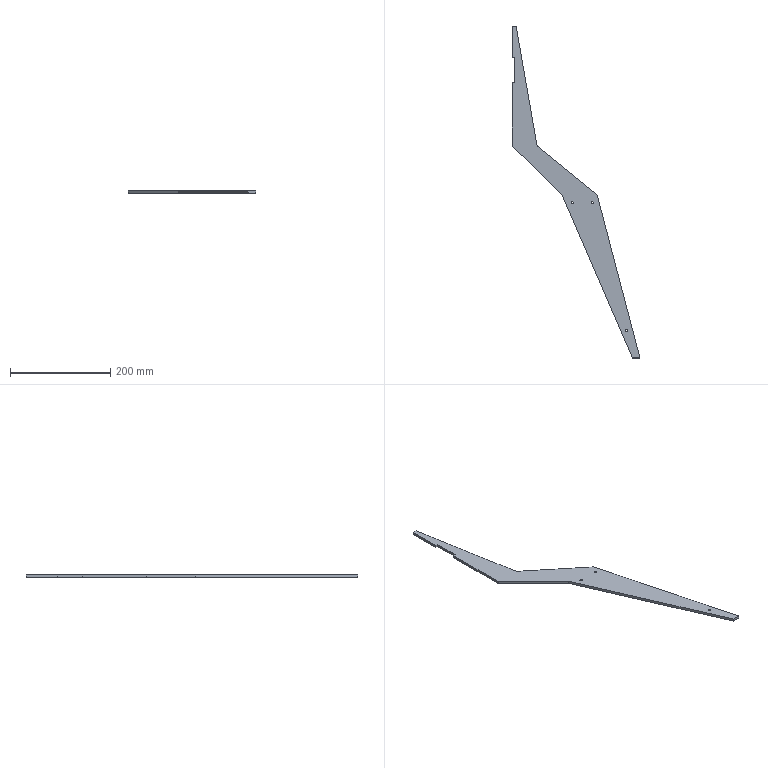Part | SolidWorks | features Cut 1, Extrusion 1, ICE 1 | 1 solid | 20 faces | box 255 x 663 x 5 mm | volume 131784 mm3 | plane 14 | cylinder 6 | commonest cylinder face diameters 4.4 x6
STEP:
#1=CARTESIAN_POINT('',(230.662,-608.,-2.5));
#2=VERTEX_POINT('',#1);
#3=CARTESIAN_POINT('',(226.262,-608.,-2.5));
#4=VERTEX_POINT('',#3);
#5=CARTESIAN_POINT('',(228.462,-608.,-2.5));
#6=DIRECTION('',(0.,0.,-1.));
#7=DIRECTION('',(-1.,0.,0.));
#8=AXIS2_PLACEMENT_3D('',#5,#6,#7);
#9=CIRCLE('',#8,2.2);
#10=EDGE_CURVE('',#2,#4,#9,.T.);
#11=ORIENTED_EDGE('',*,*,#10,.T.);
#12=CARTESIAN_POINT('',(226.262,-608.,2.5));
#13=VERTEX_POINT('',#12);
#14=CARTESIAN_POINT('',(226.262,-608.,-7.5));
#15=DIRECTION('',(0.,0.,1.));
#16=VECTOR('',#15,1000.);
#17=LINE('',#14,#16);
#18=EDGE_CURVE('',#4,#13,#17,.T.);
#19=ORIENTED_EDGE('',*,*,#18,.T.);
#20=CARTESIAN_POINT('',(230.662,-608.,2.5));
#21=VERTEX_POINT('',#20);
#22=CARTESIAN_POINT('',(228.462,-608.,2.5));
#23=DIRECTION('',(0.,0.,1.));
#24=DIRECTION('',(1.,0.,0.));
#25=AXIS2_PLACEMENT_3D('',#22,#23,#24);
#26=CIRCLE('',#25,2.2);
#27=EDGE_CURVE('',#13,#21,#26,.T.);
#28=ORIENTED_EDGE('',*,*,#27,.T.);
#29=CARTESIAN_POINT('',(230.662,-608.,-7.5));
#30=DIRECTION('',(0.,0.,1.));
#31=VECTOR('',#30,1000.);
#32=LINE('',#29,#31);
#33=EDGE_CURVE('',#2,#21,#32,.T.);
#34=ORIENTED_EDGE('',*,*,#33,.F.);
#35=EDGE_LOOP('',(#11,#19,#28,#34));
#36=FACE_OUTER_BOUND('',#35,.T.);
#37=CARTESIAN_POINT('',(228.462,-608.,-7.5));
#38=DIRECTION('',(0.,0.,1.));
#39=DIRECTION('',(1.,0.,0.));
#40=AXIS2_PLACEMENT_3D('',#37,#38,#39);
#41=CYLINDRICAL_SURFACE('',#40,2.2);
#42=ADVANCED_FACE('',(#36),#41,.F.);
#43=CARTESIAN_POINT('',(122.392,-353.,-2.5));
#44=VERTEX_POINT('',#43);
#45=CARTESIAN_POINT('',(117.992,-353.,-2.5));
#46=VERTEX_POINT('',#45);
#47=CARTESIAN_POINT('',(120.192,-353.,-2.5));
#48=DIRECTION('',(0.,0.,-1.));
#49=DIRECTION('',(-1.,0.,0.));
#50=AXIS2_PLACEMENT_3D('',#47,#48,#49);
#51=CIRCLE('',#50,2.2);
#52=EDGE_CURVE('',#44,#46,#51,.T.);
#53=ORIENTED_EDGE('',*,*,#52,.T.);
#54=CARTESIAN_POINT('',(117.992,-353.,2.5));
#55=VERTEX_POINT('',#54);
#56=CARTESIAN_POINT('',(117.992,-353.,-7.5));
#57=DIRECTION('',(0.,0.,1.));
#58=VECTOR('',#57,1000.);
#59=LINE('',#56,#58);
#60=EDGE_CURVE('',#46,#55,#59,.T.);
#61=ORIENTED_EDGE('',*,*,#60,.T.);
#62=CARTESIAN_POINT('',(122.392,-353.,2.5));
#63=VERTEX_POINT('',#62);
#64=CARTESIAN_POINT('',(120.192,-353.,2.5));
#65=DIRECTION('',(0.,0.,1.));
#66=DIRECTION('',(1.,0.,0.));
#67=AXIS2_PLACEMENT_3D('',#64,#65,#66);
#68=CIRCLE('',#67,2.2);
#69=EDGE_CURVE('',#55,#63,#68,.T.);
#70=ORIENTED_EDGE('',*,*,#69,.T.);
#71=CARTESIAN_POINT('',(122.392,-353.,-7.5));
#72=DIRECTION('',(0.,0.,1.));
#73=VECTOR('',#72,1000.);
#74=LINE('',#71,#73);
#75=EDGE_CURVE('',#44,#63,#74,.T.);
#76=ORIENTED_EDGE('',*,*,#75,.F.);
#77=EDGE_LOOP('',(#53,#61,#70,#76));
#78=FACE_OUTER_BOUND('',#77,.T.);
#79=CARTESIAN_POINT('',(120.192,-353.,-7.5));
#80=DIRECTION('',(0.,0.,1.));
#81=DIRECTION('',(1.,0.,0.));
#82=AXIS2_PLACEMENT_3D('',#79,#80,#81);
#83=CYLINDRICAL_SURFACE('',#82,2.2);
#84=ADVANCED_FACE('',(#78),#83,.F.);
#85=CARTESIAN_POINT('',(162.392,-353.,-2.5));
#86=VERTEX_POINT('',#85);
#87=CARTESIAN_POINT('',(157.992,-353.,-2.5));
#88=VERTEX_POINT('',#87);
#89=CARTESIAN_POINT('',(160.192,-353.,-2.5));
#90=DIRECTION('',(0.,0.,-1.));
#91=DIRECTION('',(-1.,0.,0.));
#92=AXIS2_PLACEMENT_3D('',#89,#90,#91);
#93=CIRCLE('',#92,2.2);
#94=EDGE_CURVE('',#86,#88,#93,.T.);
#95=ORIENTED_EDGE('',*,*,#94,.T.);
#96=CARTESIAN_POINT('',(157.992,-353.,2.5));
#97=VERTEX_POINT('',#96);
#98=CARTESIAN_POINT('',(157.992,-353.,-7.5));
#99=DIRECTION('',(0.,0.,1.));
#100=VECTOR('',#99,1000.);
#101=LINE('',#98,#100);
#102=EDGE_CURVE('',#88,#97,#101,.T.);
#103=ORIENTED_EDGE('',*,*,#102,.T.);
#104=CARTESIAN_POINT('',(162.392,-353.,2.5));
#105=VERTEX_POINT('',#104);
#106=CARTESIAN_POINT('',(160.192,-353.,2.5));
#107=DIRECTION('',(0.,0.,1.));
#108=DIRECTION('',(1.,0.,0.));
#109=AXIS2_PLACEMENT_3D('',#106,#107,#108);
#110=CIRCLE('',#109,2.2);
#111=EDGE_CURVE('',#97,#105,#110,.T.);
#112=ORIENTED_EDGE('',*,*,#111,.T.);
#113=CARTESIAN_POINT('',(162.392,-353.,-7.5));
#114=DIRECTION('',(0.,0.,1.));
#115=VECTOR('',#114,1000.);
#116=LINE('',#113,#115);
#117=EDGE_CURVE('',#86,#105,#116,.T.);
#118=ORIENTED_EDGE('',*,*,#117,.F.);
#119=EDGE_LOOP('',(#95,#103,#112,#118));
#120=FACE_OUTER_BOUND('',#119,.T.);
#121=CARTESIAN_POINT('',(160.192,-353.,-7.5));
#122=DIRECTION('',(0.,0.,1.));
#123=DIRECTION('',(1.,0.,0.));
#124=AXIS2_PLACEMENT_3D('',#121,#122,#123);
#125=CYLINDRICAL_SURFACE('',#124,2.2);
#126=ADVANCED_FACE('',(#120),#125,.F.);
#127=CARTESIAN_POINT('',(0.,0.,-2.5));
#128=VERTEX_POINT('',#127);
#129=CARTESIAN_POINT('',(0.,-63.,-2.5));
#130=VERTEX_POINT('',#129);
#131=CARTESIAN_POINT('',(0.,-63.,-2.5));
#132=DIRECTION('',(0.,-1.,0.));
#133=VECTOR('',#132,1000.);
#134=LINE('',#131,#133);
#135=EDGE_CURVE('',#128,#130,#134,.T.);
#136=ORIENTED_EDGE('',*,*,#135,.T.);
#137=CARTESIAN_POINT('',(0.,-63.,2.5));
#138=VERTEX_POINT('',#137);
#139=CARTESIAN_POINT('',(0.,-63.,2.5));
#140=DIRECTION('',(0.,0.,-1.));
#141=VECTOR('',#140,1000.);
#142=LINE('',#139,#141);
#143=EDGE_CURVE('',#138,#130,#142,.T.);
#144=ORIENTED_EDGE('',*,*,#143,.F.);
#145=CARTESIAN_POINT('',(0.,0.,2.5));
#146=VERTEX_POINT('',#145);
#147=CARTESIAN_POINT('',(0.,-63.,2.5));
#148=DIRECTION('',(0.,-1.,0.));
#149=VECTOR('',#148,1000.);
#150=LINE('',#147,#149);
#151=EDGE_CURVE('',#146,#138,#150,.T.);
#152=ORIENTED_EDGE('',*,*,#151,.F.);
#153=CARTESIAN_POINT('',(0.,0.,2.5));
#154=DIRECTION('',(0.,0.,-1.));
#155=VECTOR('',#154,1000.);
#156=LINE('',#153,#155);
#157=EDGE_CURVE('',#146,#128,#156,.T.);
#158=ORIENTED_EDGE('',*,*,#157,.T.);
#159=EDGE_LOOP('',(#136,#144,#152,#158));
#160=FACE_OUTER_BOUND('',#159,.T.);
#161=CARTESIAN_POINT('',(0.,-63.,2.5));
#162=DIRECTION('',(1.,0.,0.));
#163=DIRECTION('',(0.,0.,-1.));
#164=AXIS2_PLACEMENT_3D('',#161,#162,#163);
#165=PLANE('',#164);
#166=ADVANCED_FACE('',(#160),#165,.F.);
#167=CARTESIAN_POINT('',(5.,-63.,-2.5));
#168=VERTEX_POINT('',#167);
#169=CARTESIAN_POINT('',(5.,-63.,-2.5));
#170=DIRECTION('',(1.,0.,0.));
#171=VECTOR('',#170,1000.);
#172=LINE('',#169,#171);
#173=EDGE_CURVE('',#130,#168,#172,.T.);
#174=ORIENTED_EDGE('',*,*,#173,.T.);
#175=CARTESIAN_POINT('',(5.,-63.,2.5));
#176=VERTEX_POINT('',#175);
#177=CARTESIAN_POINT('',(5.,-63.,2.5));
#178=DIRECTION('',(0.,0.,-1.));
#179=VECTOR('',#178,1000.);
#180=LINE('',#177,#179);
#181=EDGE_CURVE('',#176,#168,#180,.T.);
#182=ORIENTED_EDGE('',*,*,#181,.F.);
#183=CARTESIAN_POINT('',(5.,-63.,2.5));
#184=DIRECTION('',(1.,0.,0.));
#185=VECTOR('',#184,1000.);
#186=LINE('',#183,#185);
#187=EDGE_CURVE('',#138,#176,#186,.T.);
#188=ORIENTED_EDGE('',*,*,#187,.F.);
#189=ORIENTED_EDGE('',*,*,#143,.T.);
#190=EDGE_LOOP('',(#174,#182,#188,#189));
#191=FACE_OUTER_BOUND('',#190,.T.);
#192=CARTESIAN_POINT('',(5.,-63.,2.5));
#193=DIRECTION('',(0.,1.,0.));
#194=DIRECTION('',(0.,0.,1.));
#195=AXIS2_PLACEMENT_3D('',#192,#193,#194);
#196=PLANE('',#195);
#197=ADVANCED_FACE('',(#191),#196,.F.);
#198=CARTESIAN_POINT('',(5.,-113.,-2.5));
#199=VERTEX_POINT('',#198);
#200=CARTESIAN_POINT('',(5.,-113.,-2.5));
#201=DIRECTION('',(0.,-1.,0.));
#202=VECTOR('',#201,1000.);
#203=LINE('',#200,#202);
#204=EDGE_CURVE('',#168,#199,#203,.T.);
#205=ORIENTED_EDGE('',*,*,#204,.T.);
#206=CARTESIAN_POINT('',(5.,-113.,2.5));
#207=VERTEX_POINT('',#206);
#208=CARTESIAN_POINT('',(5.,-113.,2.5));
#209=DIRECTION('',(0.,0.,-1.));
#210=VECTOR('',#209,1000.);
#211=LINE('',#208,#210);
#212=EDGE_CURVE('',#207,#199,#211,.T.);
#213=ORIENTED_EDGE('',*,*,#212,.F.);
#214=CARTESIAN_POINT('',(5.,-113.,2.5));
#215=DIRECTION('',(0.,-1.,0.));
#216=VECTOR('',#215,1000.);
#217=LINE('',#214,#216);
#218=EDGE_CURVE('',#176,#207,#217,.T.);
#219=ORIENTED_EDGE('',*,*,#218,.F.);
#220=ORIENTED_EDGE('',*,*,#181,.T.);
#221=EDGE_LOOP('',(#205,#213,#219,#220));
#222=FACE_OUTER_BOUND('',#221,.T.);
#223=CARTESIAN_POINT('',(5.,-113.,2.5));
#224=DIRECTION('',(1.,0.,0.));
#225=DIRECTION('',(0.,0.,-1.));
#226=AXIS2_PLACEMENT_3D('',#223,#224,#225);
#227=PLANE('',#226);
#228=ADVANCED_FACE('',(#222),#227,.F.);
#229=CARTESIAN_POINT('',(0.,-113.,-2.5));
#230=VERTEX_POINT('',#229);
#231=CARTESIAN_POINT('',(0.,-113.,-2.5));
#232=DIRECTION('',(-1.,0.,0.));
#233=VECTOR('',#232,1000.);
#234=LINE('',#231,#233);
#235=EDGE_CURVE('',#199,#230,#234,.T.);
#236=ORIENTED_EDGE('',*,*,#235,.T.);
#237=CARTESIAN_POINT('',(0.,-113.,2.5));
#238=VERTEX_POINT('',#237);
#239=CARTESIAN_POINT('',(0.,-113.,2.5));
#240=DIRECTION('',(0.,0.,-1.));
#241=VECTOR('',#240,1000.);
#242=LINE('',#239,#241);
#243=EDGE_CURVE('',#238,#230,#242,.T.);
#244=ORIENTED_EDGE('',*,*,#243,.F.);
#245=CARTESIAN_POINT('',(0.,-113.,2.5));
#246=DIRECTION('',(-1.,0.,0.));
#247=VECTOR('',#246,1000.);
#248=LINE('',#245,#247);
#249=EDGE_CURVE('',#207,#238,#248,.T.);
#250=ORIENTED_EDGE('',*,*,#249,.F.);
#251=ORIENTED_EDGE('',*,*,#212,.T.);
#252=EDGE_LOOP('',(#236,#244,#250,#251));
#253=FACE_OUTER_BOUND('',#252,.T.);
#254=CARTESIAN_POINT('',(0.,-113.,2.5));
#255=DIRECTION('',(0.,-1.,0.));
#256=DIRECTION('',(0.,0.,-1.));
#257=AXIS2_PLACEMENT_3D('',#254,#255,#256);
#258=PLANE('',#257);
#259=ADVANCED_FACE('',(#253),#258,.F.);
#260=CARTESIAN_POINT('',(0.,-240.,-2.5));
#261=VERTEX_POINT('',#260);
#262=CARTESIAN_POINT('',(0.,-240.,-2.5));
#263=DIRECTION('',(0.,-1.,0.));
#264=VECTOR('',#263,1000.);
#265=LINE('',#262,#264);
#266=EDGE_CURVE('',#230,#261,#265,.T.);
#267=ORIENTED_EDGE('',*,*,#266,.T.);
#268=CARTESIAN_POINT('',(0.,-240.,2.5));
#269=VERTEX_POINT('',#268);
#270=CARTESIAN_POINT('',(0.,-240.,2.5));
#271=DIRECTION('',(0.,0.,-1.));
#272=VECTOR('',#271,1000.);
#273=LINE('',#270,#272);
#274=EDGE_CURVE('',#269,#261,#273,.T.);
#275=ORIENTED_EDGE('',*,*,#274,.F.);
#276=CARTESIAN_POINT('',(0.,-240.,2.5));
#277=DIRECTION('',(0.,-1.,0.));
#278=VECTOR('',#277,1000.);
#279=LINE('',#276,#278);
#280=EDGE_CURVE('',#238,#269,#279,.T.);
#281=ORIENTED_EDGE('',*,*,#280,.F.);
#282=ORIENTED_EDGE('',*,*,#243,.T.);
#283=EDGE_LOOP('',(#267,#275,#281,#282));
#284=FACE_OUTER_BOUND('',#283,.T.);
#285=CARTESIAN_POINT('',(0.,-240.,2.5));
#286=DIRECTION('',(1.,0.,0.));
#287=DIRECTION('',(0.,0.,-1.));
#288=AXIS2_PLACEMENT_3D('',#285,#286,#287);
#289=PLANE('',#288);
#290=ADVANCED_FACE('',(#284),#289,.F.);
#291=CARTESIAN_POINT('',(100.,-338.,-2.5));
#292=VERTEX_POINT('',#291);
#293=CARTESIAN_POINT('',(100.,-338.,-2.5));
#294=DIRECTION('',(0.7142,-0.6999,0.));
#295=VECTOR('',#294,1000.);
#296=LINE('',#293,#295);
#297=EDGE_CURVE('',#261,#292,#296,.T.);
#298=ORIENTED_EDGE('',*,*,#297,.T.);
#299=CARTESIAN_POINT('',(100.,-338.,2.5));
#300=VERTEX_POINT('',#299);
#301=CARTESIAN_POINT('',(100.,-338.,2.5));
#302=DIRECTION('',(0.,0.,-1.));
#303=VECTOR('',#302,1000.);
#304=LINE('',#301,#303);
#305=EDGE_CURVE('',#300,#292,#304,.T.);
#306=ORIENTED_EDGE('',*,*,#305,.F.);
#307=CARTESIAN_POINT('',(100.,-338.,2.5));
#308=DIRECTION('',(0.7142,-0.6999,0.));
#309=VECTOR('',#308,1000.);
#310=LINE('',#307,#309);
#311=EDGE_CURVE('',#269,#300,#310,.T.);
#312=ORIENTED_EDGE('',*,*,#311,.F.);
#313=ORIENTED_EDGE('',*,*,#274,.T.);
#314=EDGE_LOOP('',(#298,#306,#312,#313));
#315=FACE_OUTER_BOUND('',#314,.T.);
#316=CARTESIAN_POINT('',(100.,-338.,2.5));
#317=DIRECTION('',(0.6999,0.7142,0.));
#318=DIRECTION('',(-0.7142,0.6999,0.));
#319=AXIS2_PLACEMENT_3D('',#316,#317,#318);
#320=PLANE('',#319);
#321=ADVANCED_FACE('',(#315),#320,.F.);
#322=CARTESIAN_POINT('',(240.,-663.,-2.5));
#323=VERTEX_POINT('',#322);
#324=CARTESIAN_POINT('',(240.,-663.,-2.5));
#325=DIRECTION('',(0.3956,-0.9184,0.));
#326=VECTOR('',#325,1000.);
#327=LINE('',#324,#326);
#328=EDGE_CURVE('',#292,#323,#327,.T.);
#329=ORIENTED_EDGE('',*,*,#328,.T.);
#330=CARTESIAN_POINT('',(240.,-663.,2.5));
#331=VERTEX_POINT('',#330);
#332=CARTESIAN_POINT('',(240.,-663.,2.5));
#333=DIRECTION('',(0.,0.,-1.));
#334=VECTOR('',#333,1000.);
#335=LINE('',#332,#334);
#336=EDGE_CURVE('',#331,#323,#335,.T.);
#337=ORIENTED_EDGE('',*,*,#336,.F.);
#338=CARTESIAN_POINT('',(240.,-663.,2.5));
#339=DIRECTION('',(0.3956,-0.9184,0.));
#340=VECTOR('',#339,1000.);
#341=LINE('',#338,#340);
#342=EDGE_CURVE('',#300,#331,#341,.T.);
#343=ORIENTED_EDGE('',*,*,#342,.F.);
#344=ORIENTED_EDGE('',*,*,#305,.T.);
#345=EDGE_LOOP('',(#329,#337,#343,#344));
#346=FACE_OUTER_BOUND('',#345,.T.);
#347=CARTESIAN_POINT('',(240.,-663.,2.5));
#348=DIRECTION('',(0.9184,0.3956,0.));
#349=DIRECTION('',(-0.3956,0.9184,0.));
#350=AXIS2_PLACEMENT_3D('',#347,#348,#349);
#351=PLANE('',#350);
#352=ADVANCED_FACE('',(#346),#351,.F.);
#353=CARTESIAN_POINT('',(255.,-663.,-2.5));
#354=VERTEX_POINT('',#353);
#355=CARTESIAN_POINT('',(255.,-663.,-2.5));
#356=DIRECTION('',(1.,0.,0.));
#357=VECTOR('',#356,1000.);
#358=LINE('',#355,#357);
#359=EDGE_CURVE('',#323,#354,#358,.T.);
#360=ORIENTED_EDGE('',*,*,#359,.T.);
#361=CARTESIAN_POINT('',(255.,-663.,2.5));
#362=VERTEX_POINT('',#361);
#363=CARTESIAN_POINT('',(255.,-663.,2.5));
#364=DIRECTION('',(0.,0.,-1.));
#365=VECTOR('',#364,1000.);
#366=LINE('',#363,#365);
#367=EDGE_CURVE('',#362,#354,#366,.T.);
#368=ORIENTED_EDGE('',*,*,#367,.F.);
#369=CARTESIAN_POINT('',(255.,-663.,2.5));
#370=DIRECTION('',(1.,0.,0.));
#371=VECTOR('',#370,1000.);
#372=LINE('',#369,#371);
#373=EDGE_CURVE('',#331,#362,#372,.T.);
#374=ORIENTED_EDGE('',*,*,#373,.F.);
#375=ORIENTED_EDGE('',*,*,#336,.T.);
#376=EDGE_LOOP('',(#360,#368,#374,#375));
#377=FACE_OUTER_BOUND('',#376,.T.);
#378=CARTESIAN_POINT('',(255.,-663.,2.5));
#379=DIRECTION('',(0.,1.,0.));
#380=DIRECTION('',(0.,0.,1.));
#381=AXIS2_PLACEMENT_3D('',#378,#379,#380);
#382=PLANE('',#381);
#383=ADVANCED_FACE('',(#377),#382,.F.);
#384=CARTESIAN_POINT('',(170.,-338.,-2.5));
#385=VERTEX_POINT('',#384);
#386=CARTESIAN_POINT('',(170.,-338.,-2.5));
#387=DIRECTION('',(-0.253,0.9675,0.));
#388=VECTOR('',#387,1000.);
#389=LINE('',#386,#388);
#390=EDGE_CURVE('',#354,#385,#389,.T.);
#391=ORIENTED_EDGE('',*,*,#390,.T.);
#392=CARTESIAN_POINT('',(170.,-338.,2.5));
#393=VERTEX_POINT('',#392);
#394=CARTESIAN_POINT('',(170.,-338.,2.5));
#395=DIRECTION('',(0.,0.,-1.));
#396=VECTOR('',#395,1000.);
#397=LINE('',#394,#396);
#398=EDGE_CURVE('',#393,#385,#397,.T.);
#399=ORIENTED_EDGE('',*,*,#398,.F.);
#400=CARTESIAN_POINT('',(170.,-338.,2.5));
#401=DIRECTION('',(-0.253,0.9675,0.));
#402=VECTOR('',#401,1000.);
#403=LINE('',#400,#402);
#404=EDGE_CURVE('',#362,#393,#403,.T.);
#405=ORIENTED_EDGE('',*,*,#404,.F.);
#406=ORIENTED_EDGE('',*,*,#367,.T.);
#407=EDGE_LOOP('',(#391,#399,#405,#406));
#408=FACE_OUTER_BOUND('',#407,.T.);
#409=CARTESIAN_POINT('',(170.,-338.,2.5));
#410=DIRECTION('',(-0.9675,-0.253,0.));
#411=DIRECTION('',(0.253,-0.9675,0.));
#412=AXIS2_PLACEMENT_3D('',#409,#410,#411);
#413=PLANE('',#412);
#414=ADVANCED_FACE('',(#408),#413,.F.);
#415=CARTESIAN_POINT('',(50.,-240.,-2.5));
#416=VERTEX_POINT('',#415);
#417=CARTESIAN_POINT('',(50.,-240.,-2.5));
#418=DIRECTION('',(-0.7745,0.6325,0.));
#419=VECTOR('',#418,1000.);
#420=LINE('',#417,#419);
#421=EDGE_CURVE('',#385,#416,#420,.T.);
#422=ORIENTED_EDGE('',*,*,#421,.T.);
#423=CARTESIAN_POINT('',(50.,-240.,2.5));
#424=VERTEX_POINT('',#423);
#425=CARTESIAN_POINT('',(50.,-240.,2.5));
#426=DIRECTION('',(0.,0.,-1.));
#427=VECTOR('',#426,1000.);
#428=LINE('',#425,#427);
#429=EDGE_CURVE('',#424,#416,#428,.T.);
#430=ORIENTED_EDGE('',*,*,#429,.F.);
#431=CARTESIAN_POINT('',(50.,-240.,2.5));
#432=DIRECTION('',(-0.7745,0.6325,0.));
#433=VECTOR('',#432,1000.);
#434=LINE('',#431,#433);
#435=EDGE_CURVE('',#393,#424,#434,.T.);
#436=ORIENTED_EDGE('',*,*,#435,.F.);
#437=ORIENTED_EDGE('',*,*,#398,.T.);
#438=EDGE_LOOP('',(#422,#430,#436,#437));
#439=FACE_OUTER_BOUND('',#438,.T.);
#440=CARTESIAN_POINT('',(50.,-240.,2.5));
#441=DIRECTION('',(-0.6325,-0.7745,0.));
#442=DIRECTION('',(0.7745,-0.6325,0.));
#443=AXIS2_PLACEMENT_3D('',#440,#441,#442);
#444=PLANE('',#443);
#445=ADVANCED_FACE('',(#439),#444,.F.);
#446=CARTESIAN_POINT('',(8.,0.,-2.5));
#447=VERTEX_POINT('',#446);
#448=CARTESIAN_POINT('',(8.,0.,-2.5));
#449=DIRECTION('',(-0.1724,0.985,0.));
#450=VECTOR('',#449,1000.);
#451=LINE('',#448,#450);
#452=EDGE_CURVE('',#416,#447,#451,.T.);
#453=ORIENTED_EDGE('',*,*,#452,.T.);
#454=CARTESIAN_POINT('',(8.,0.,2.5));
#455=VERTEX_POINT('',#454);
#456=CARTESIAN_POINT('',(8.,0.,2.5));
#457=DIRECTION('',(0.,0.,-1.));
#458=VECTOR('',#457,1000.);
#459=LINE('',#456,#458);
#460=EDGE_CURVE('',#455,#447,#459,.T.);
#461=ORIENTED_EDGE('',*,*,#460,.F.);
#462=CARTESIAN_POINT('',(8.,0.,2.5));
#463=DIRECTION('',(-0.1724,0.985,0.));
#464=VECTOR('',#463,1000.);
#465=LINE('',#462,#464);
#466=EDGE_CURVE('',#424,#455,#465,.T.);
#467=ORIENTED_EDGE('',*,*,#466,.F.);
#468=ORIENTED_EDGE('',*,*,#429,.T.);
#469=EDGE_LOOP('',(#453,#461,#467,#468));
#470=FACE_OUTER_BOUND('',#469,.T.);
#471=CARTESIAN_POINT('',(8.,0.,2.5));
#472=DIRECTION('',(-0.985,-0.1724,0.));
#473=DIRECTION('',(0.1724,-0.985,0.));
#474=AXIS2_PLACEMENT_3D('',#471,#472,#473);
#475=PLANE('',#474);
#476=ADVANCED_FACE('',(#470),#475,.F.);
#477=CARTESIAN_POINT('',(0.,0.,-2.5));
#478=DIRECTION('',(-1.,0.,0.));
#479=VECTOR('',#478,1000.);
#480=LINE('',#477,#479);
#481=EDGE_CURVE('',#447,#128,#480,.T.);
#482=ORIENTED_EDGE('',*,*,#481,.T.);
#483=ORIENTED_EDGE('',*,*,#157,.F.);
#484=CARTESIAN_POINT('',(0.,0.,2.5));
#485=DIRECTION('',(-1.,0.,0.));
#486=VECTOR('',#485,1000.);
#487=LINE('',#484,#486);
#488=EDGE_CURVE('',#455,#146,#487,.T.);
#489=ORIENTED_EDGE('',*,*,#488,.F.);
#490=ORIENTED_EDGE('',*,*,#460,.T.);
#491=EDGE_LOOP('',(#482,#483,#489,#490));
#492=FACE_OUTER_BOUND('',#491,.T.);
#493=CARTESIAN_POINT('',(0.,0.,2.5));
#494=DIRECTION('',(0.,-1.,0.));
#495=DIRECTION('',(0.,0.,-1.));
#496=AXIS2_PLACEMENT_3D('',#493,#494,#495);
#497=PLANE('',#496);
#498=ADVANCED_FACE('',(#492),#497,.F.);
#499=CARTESIAN_POINT('',(228.462,-608.,2.5));
#500=DIRECTION('',(0.,0.,1.));
#501=DIRECTION('',(1.,0.,0.));
#502=AXIS2_PLACEMENT_3D('',#499,#500,#501);
#503=CIRCLE('',#502,2.2);
#504=EDGE_CURVE('',#21,#13,#503,.T.);
#505=ORIENTED_EDGE('',*,*,#504,.F.);
#506=ORIENTED_EDGE('',*,*,#27,.F.);
#507=EDGE_LOOP('',(#505,#506));
#508=FACE_BOUND('',#507,.T.);
#509=CARTESIAN_POINT('',(120.192,-353.,2.5));
#510=DIRECTION('',(0.,0.,1.));
#511=DIRECTION('',(1.,0.,0.));
#512=AXIS2_PLACEMENT_3D('',#509,#510,#511);
#513=CIRCLE('',#512,2.2);
#514=EDGE_CURVE('',#63,#55,#513,.T.);
#515=ORIENTED_EDGE('',*,*,#514,.F.);
#516=ORIENTED_EDGE('',*,*,#69,.F.);
#517=EDGE_LOOP('',(#515,#516));
#518=FACE_BOUND('',#517,.T.);
#519=CARTESIAN_POINT('',(160.192,-353.,2.5));
#520=DIRECTION('',(0.,0.,1.));
#521=DIRECTION('',(1.,0.,0.));
#522=AXIS2_PLACEMENT_3D('',#519,#520,#521);
#523=CIRCLE('',#522,2.2);
#524=EDGE_CURVE('',#105,#97,#523,.T.);
#525=ORIENTED_EDGE('',*,*,#524,.F.);
#526=ORIENTED_EDGE('',*,*,#111,.F.);
#527=EDGE_LOOP('',(#525,#526));
#528=FACE_BOUND('',#527,.T.);
#529=ORIENTED_EDGE('',*,*,#151,.T.);
#530=ORIENTED_EDGE('',*,*,#187,.T.);
#531=ORIENTED_EDGE('',*,*,#218,.T.);
#532=ORIENTED_EDGE('',*,*,#249,.T.);
#533=ORIENTED_EDGE('',*,*,#280,.T.);
#534=ORIENTED_EDGE('',*,*,#311,.T.);
#535=ORIENTED_EDGE('',*,*,#342,.T.);
#536=ORIENTED_EDGE('',*,*,#373,.T.);
#537=ORIENTED_EDGE('',*,*,#404,.T.);
#538=ORIENTED_EDGE('',*,*,#435,.T.);
#539=ORIENTED_EDGE('',*,*,#466,.T.);
#540=ORIENTED_EDGE('',*,*,#488,.T.);
#541=EDGE_LOOP('',(#529,#530,#531,#532,#533,#534,#535,#536,#537,#538,#539,#540));
#542=FACE_OUTER_BOUND('',#541,.T.);
#543=CARTESIAN_POINT('',(0.,0.,2.5));
#544=DIRECTION('',(0.,0.,-1.));
#545=DIRECTION('',(-1.,0.,0.));
#546=AXIS2_PLACEMENT_3D('',#543,#544,#545);
#547=PLANE('',#546);
#548=ADVANCED_FACE('',(#508,#518,#528,#542),#547,.F.);
#549=ORIENTED_EDGE('',*,*,#10,.F.);
#550=CARTESIAN_POINT('',(228.462,-608.,-2.5));
#551=DIRECTION('',(0.,0.,-1.));
#552=DIRECTION('',(-1.,0.,0.));
#553=AXIS2_PLACEMENT_3D('',#550,#551,#552);
#554=CIRCLE('',#553,2.2);
#555=EDGE_CURVE('',#4,#2,#554,.T.);
#556=ORIENTED_EDGE('',*,*,#555,.F.);
#557=EDGE_LOOP('',(#549,#556));
#558=FACE_BOUND('',#557,.T.);
#559=ORIENTED_EDGE('',*,*,#52,.F.);
#560=CARTESIAN_POINT('',(120.192,-353.,-2.5));
#561=DIRECTION('',(0.,0.,-1.));
#562=DIRECTION('',(-1.,0.,0.));
#563=AXIS2_PLACEMENT_3D('',#560,#561,#562);
#564=CIRCLE('',#563,2.2);
#565=EDGE_CURVE('',#46,#44,#564,.T.);
#566=ORIENTED_EDGE('',*,*,#565,.F.);
#567=EDGE_LOOP('',(#559,#566));
#568=FACE_BOUND('',#567,.T.);
#569=ORIENTED_EDGE('',*,*,#94,.F.);
#570=CARTESIAN_POINT('',(160.192,-353.,-2.5));
#571=DIRECTION('',(0.,0.,-1.));
#572=DIRECTION('',(-1.,0.,0.));
#573=AXIS2_PLACEMENT_3D('',#570,#571,#572);
#574=CIRCLE('',#573,2.2);
#575=EDGE_CURVE('',#88,#86,#574,.T.);
#576=ORIENTED_EDGE('',*,*,#575,.F.);
#577=EDGE_LOOP('',(#569,#576));
#578=FACE_BOUND('',#577,.T.);
#579=ORIENTED_EDGE('',*,*,#135,.F.);
#580=ORIENTED_EDGE('',*,*,#481,.F.);
#581=ORIENTED_EDGE('',*,*,#452,.F.);
#582=ORIENTED_EDGE('',*,*,#421,.F.);
#583=ORIENTED_EDGE('',*,*,#390,.F.);
#584=ORIENTED_EDGE('',*,*,#359,.F.);
#585=ORIENTED_EDGE('',*,*,#328,.F.);
#586=ORIENTED_EDGE('',*,*,#297,.F.);
#587=ORIENTED_EDGE('',*,*,#266,.F.);
#588=ORIENTED_EDGE('',*,*,#235,.F.);
#589=ORIENTED_EDGE('',*,*,#204,.F.);
#590=ORIENTED_EDGE('',*,*,#173,.F.);
#591=EDGE_LOOP('',(#579,#580,#581,#582,#583,#584,#585,#586,#587,#588,#589,#590));
#592=FACE_OUTER_BOUND('',#591,.T.);
#593=CARTESIAN_POINT('',(0.,0.,-2.5));
#594=DIRECTION('',(0.,0.,-1.));
#595=DIRECTION('',(-1.,0.,0.));
#596=AXIS2_PLACEMENT_3D('',#593,#594,#595);
#597=PLANE('',#596);
#598=ADVANCED_FACE('',(#558,#568,#578,#592),#597,.T.);
#599=ORIENTED_EDGE('',*,*,#102,.F.);
#600=ORIENTED_EDGE('',*,*,#575,.T.);
#601=ORIENTED_EDGE('',*,*,#117,.T.);
#602=ORIENTED_EDGE('',*,*,#524,.T.);
#603=EDGE_LOOP('',(#599,#600,#601,#602));
#604=FACE_OUTER_BOUND('',#603,.T.);
#605=CARTESIAN_POINT('',(160.192,-353.,-7.5));
#606=DIRECTION('',(0.,0.,1.));
#607=DIRECTION('',(1.,0.,0.));
#608=AXIS2_PLACEMENT_3D('',#605,#606,#607);
#609=CYLINDRICAL_SURFACE('',#608,2.2);
#610=ADVANCED_FACE('',(#604),#609,.F.);
#611=ORIENTED_EDGE('',*,*,#60,.F.);
#612=ORIENTED_EDGE('',*,*,#565,.T.);
#613=ORIENTED_EDGE('',*,*,#75,.T.);
#614=ORIENTED_EDGE('',*,*,#514,.T.);
#615=EDGE_LOOP('',(#611,#612,#613,#614));
#616=FACE_OUTER_BOUND('',#615,.T.);
#617=CARTESIAN_POINT('',(120.192,-353.,-7.5));
#618=DIRECTION('',(0.,0.,1.));
#619=DIRECTION('',(1.,0.,0.));
#620=AXIS2_PLACEMENT_3D('',#617,#618,#619);
#621=CYLINDRICAL_SURFACE('',#620,2.2);
#622=ADVANCED_FACE('',(#616),#621,.F.);
#623=ORIENTED_EDGE('',*,*,#18,.F.);
#624=ORIENTED_EDGE('',*,*,#555,.T.);
#625=ORIENTED_EDGE('',*,*,#33,.T.);
#626=ORIENTED_EDGE('',*,*,#504,.T.);
#627=EDGE_LOOP('',(#623,#624,#625,#626));
#628=FACE_OUTER_BOUND('',#627,.T.);
#629=CARTESIAN_POINT('',(228.462,-608.,-7.5));
#630=DIRECTION('',(0.,0.,1.));
#631=DIRECTION('',(1.,0.,0.));
#632=AXIS2_PLACEMENT_3D('',#629,#630,#631);
#633=CYLINDRICAL_SURFACE('',#632,2.2);
#634=ADVANCED_FACE('',(#628),#633,.F.);
#635=CLOSED_SHELL('',(#42,#84,#126,#166,#197,#228,#259,#290,#321,#352,#383,#414,#445,#476,#498,#548,#598,#610,#622,#634));
#636=MANIFOLD_SOLID_BREP('',#635);
#637=CARTESIAN_POINT('',(0.,0.,0.));
#638=DIRECTION('',(0.,0.,1.));
#639=DIRECTION('',(1.,0.,0.));
#640=AXIS2_PLACEMENT_3D('',#637,#638,#639);
#641=(LENGTH_UNIT()NAMED_UNIT(*)SI_UNIT(.MILLI.,.METRE.));
#642=UNCERTAINTY_MEASURE_WITH_UNIT(LENGTH_MEASURE(0.00001),#641,'','');
#643=(NAMED_UNIT(*)PLANE_ANGLE_UNIT()SI_UNIT($,.RADIAN.));
#644=(NAMED_UNIT(*)SI_UNIT($,.STERADIAN.)SOLID_ANGLE_UNIT());
#645=(GEOMETRIC_REPRESENTATION_CONTEXT(3)GLOBAL_UNCERTAINTY_ASSIGNED_CONTEXT((#642))GLOBAL_UNIT_ASSIGNED_CONTEXT((#641,#643,#644))REPRESENTATION_CONTEXT('',''));
#646=ADVANCED_BREP_SHAPE_REPRESENTATION('',(#636,#640),#645);